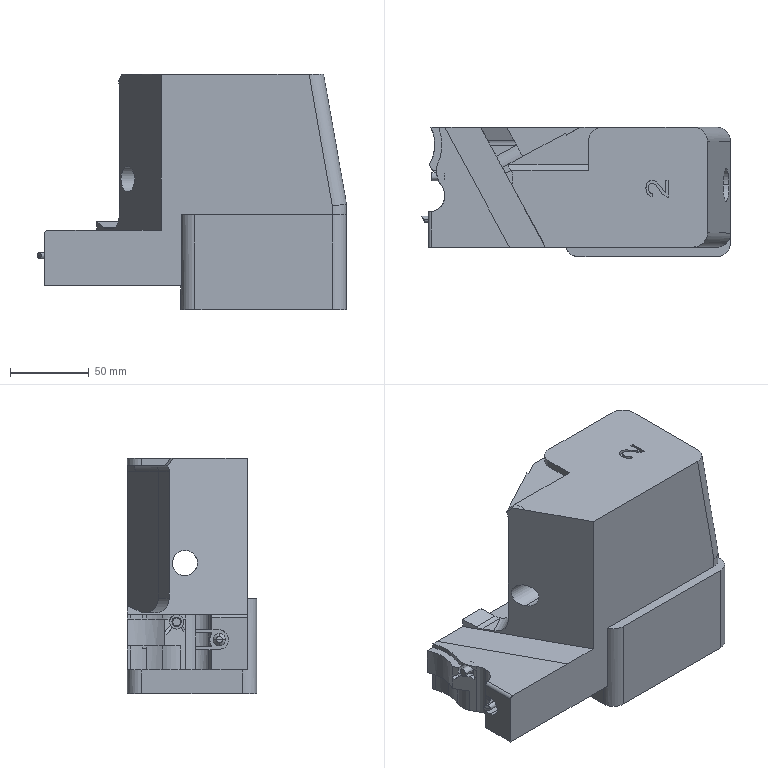Part | Creo | 1 solid | 120 faces | box 195.785 x 81.996 x 149.057 mm | volume 1520829 mm3 | plane 50 | cylinder 48 | other 12 | spline 8 | cone 2 | commonest cylinder face diameters 18 x8 1.005 x3 4.02 x3 5.025 x2 9.045 x2 14.768 x2